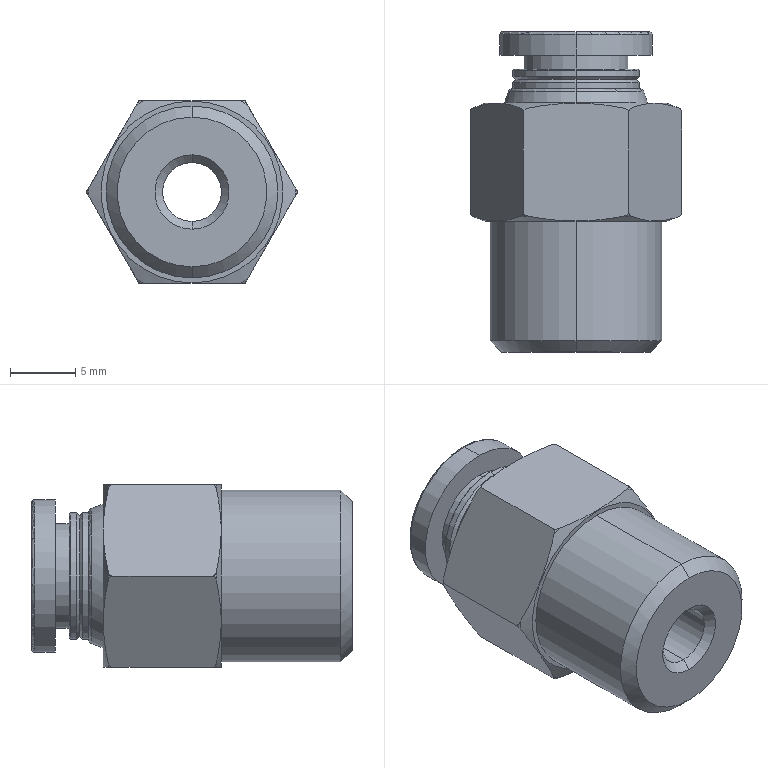Part | NX | features BREP 1 | 1 solid | 62 faces | box 16.166 x 24.5 x 14 mm | volume 2707 mm3 | torus 18 | cone 16 | cylinder 14 | plane 14 | commonest cylinder face diameters 9.7 x4 4.5 x2 6 x2 8 x2 11.7 x2 13.157 x2